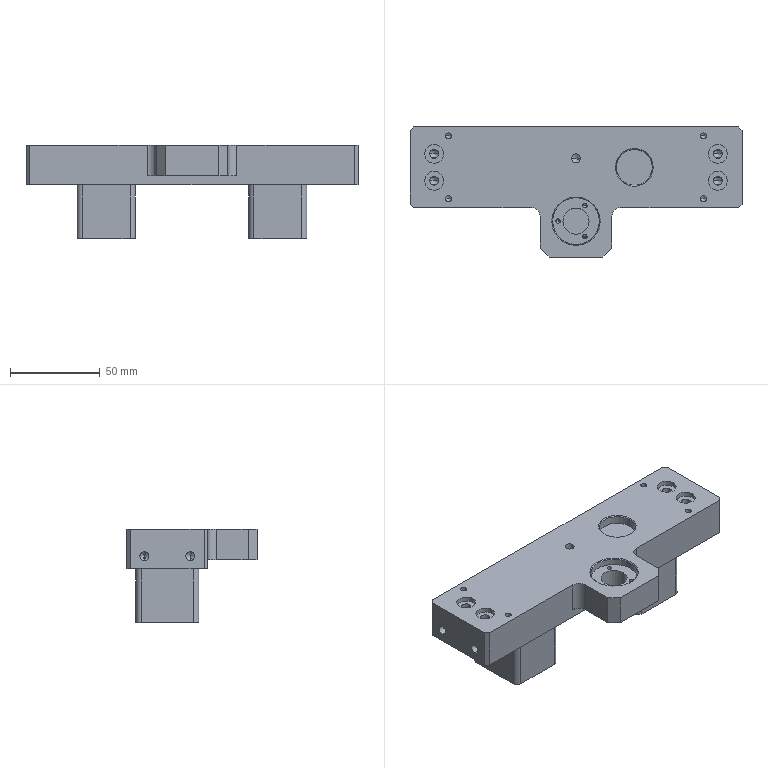NC program | NX | posted with a generic post | part box 185 x 72.5 x 52 mm
Lines 1 to 56 of 6926:
N10 G17 G21 G94 G90
(FLOOR_WALL_COPY , TOOL : D80)
N12 T19 M6
N14 G54
N16 G17 G0 G90 X142.5 Y-41.247 S6500 M3
N18 G43 Z30. H19
N20 Z3.
N22 G94 G1 Z0. F1500.
N24 X137.5
N26 X-137.5
N28 Y9.25
N30 X137.5
N32 X142.5
N34 Z3.
N36 G0 Z30.
N38 M5
(DRILLING_COPY_1 , TOOL : D6A45)
N40 T01 M6
N42 G54
N44 G17 G0 G90 X35.75 Y-26.5 S5000 M3
N46 G43 Z30. H1
N48 G94 G81 G98 Z-2.2 F350. R3.
N50 X59.75
N52 Y-1.
N54 X35.75
N56 X-35.75
N58 X-59.75
N60 Y-26.5
N62 X-35.75
N64 G80
N66 G0 X-35.75 Y-26.5 Z30.
N68 M5
(DRILLING_COPY_COPY , TOOL : 4.2ZT)
N70 T04 M6
N72 G54
N74 G17 G0 G90 X35.75 Y-26.5 S1516 M3
N76 G43 Z30. H4
N78 G94 G83 G98 Z-38.405 F180. Q2. R3.
N80 X59.75
N82 Y-1.
N84 X35.75
N86 X-35.75
N88 X-59.75
N90 Y-26.5
N92 X-35.75
N94 G80
N96 G0 X-35.75 Y-26.5 Z30.
N98 M5